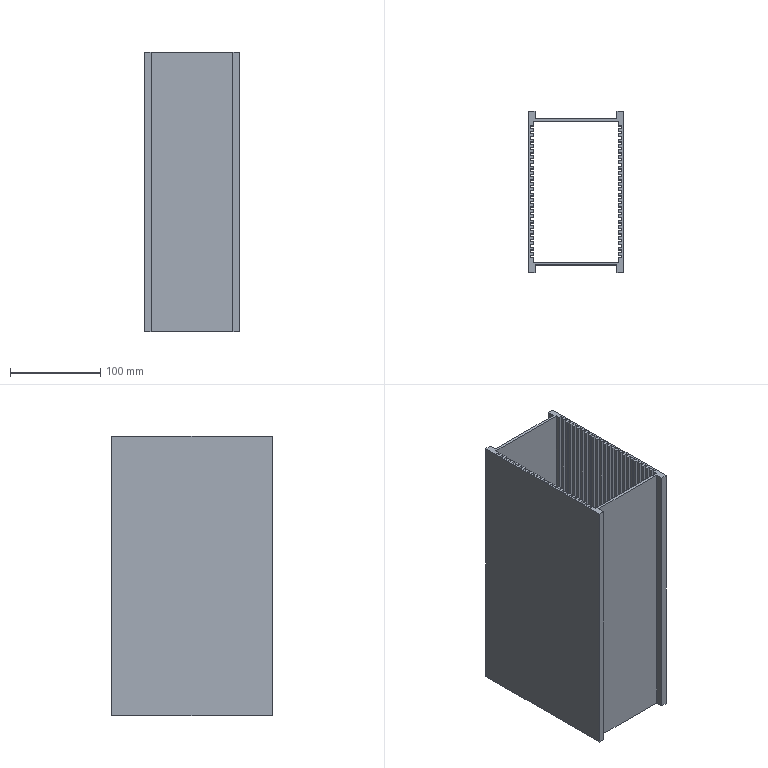Part | NX | features BREP 1 | 1 solid | 218 faces | box 105 x 178.5 x 310 mm | volume 587140 mm3 | plane 218